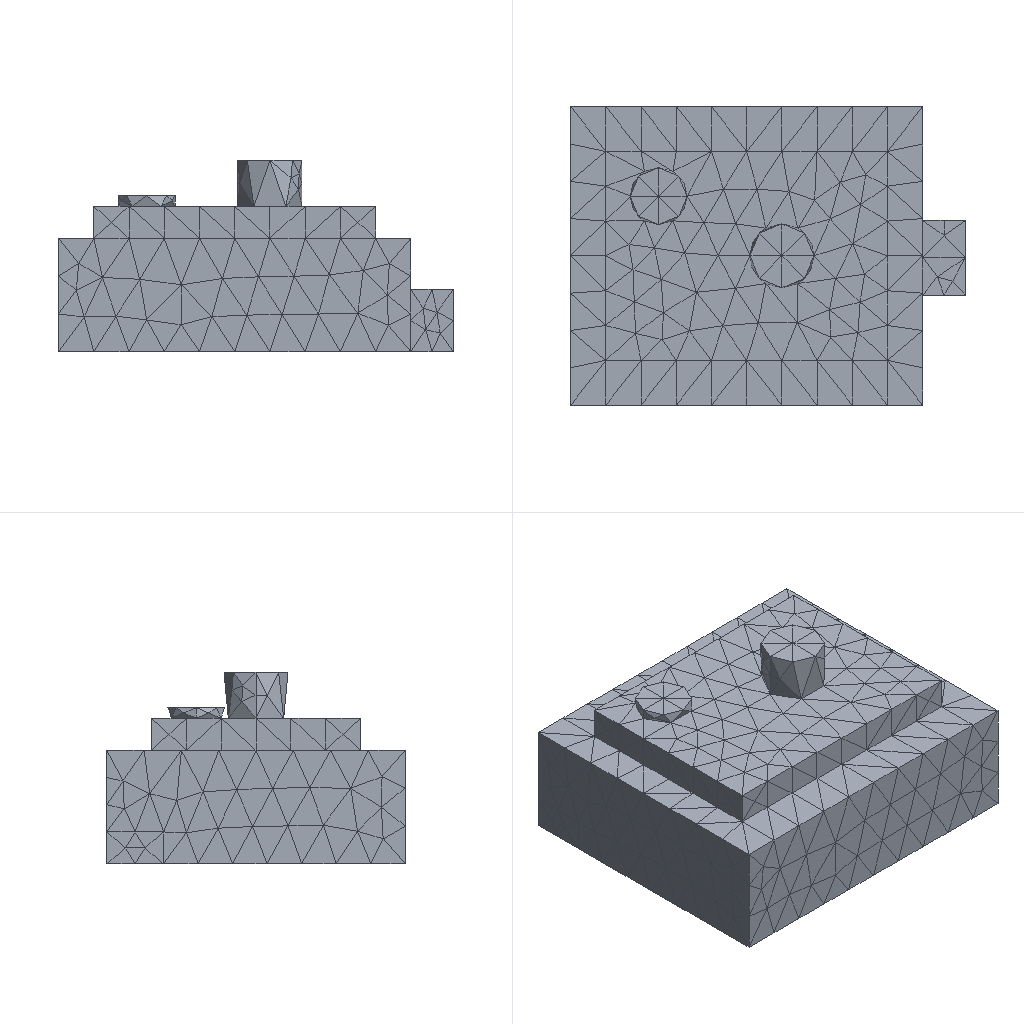Simulation study | ansys mapdl
Set-up summary:
category,name,step,type,value,unit,region
solver,ansys_mapdl
units,mm-N-s-tonne (MPa),,inferred,E=210000 density=
analysis,model,,static
mesh,nodes,,,4549
mesh,elements,,,2727
element_type,SOLID187,,,2727
material,mat 1,,E,210000
material,mat 1,,nu,0.3
load,,model,body load temp,,,all
load,,model,force,"1000 [dir=(0, 0, -1) n=148]",,node list
bc,,model,fixed,"[dofs=UX,UY,UZ n=4913]",,node list
Ansys APDL input file, long lists of numbers shortened:
/COM,ANSYS RELEASE 2026 R1           BUILD 26.1      UP20260202       09:08:28
/PREP7
/NOPR
/TITLE,2
ANTYPE, 0
*IF,_CDRDOFF,EQ,1,THEN     !if solid model was read in
_CDRDOFF=             !reset flag, numoffs already performed
*ELSE              !offset database for the following FE model
NUMOFF,NODE,     4549
NUMOFF,ELEM,     2727
NUMOFF,MAT ,        1
NUMOFF,TYPE,        1
*ENDIF
*SET,_RETURN ,  0.
*SET,_STATUS ,  0.
*SET,_UIQR   ,  148.
*SET,__FLOATPARAMETER__,  4549.
DOF,DELETE
ETBLOCK,        1,        1
(2i9,19a9)
        1      187        0        0        0        0        0        0        0        0        0        0        0        0        0        0        0        0        0        0        0
       -1
NBLOCK,6,SOLID,      4549,      4549
(3i9,6e21.13e3)
        1        0        0-3.3550000000000E+001 4.2000000000000E+001 9.0000000000000E+000
! (4548 more lines like these left out)
N,UNBL,LOC,       -1,
EBLOCK,19,SOLID,      2727,      2727
(19i10)
         1         1         1         1         0         0         0         0        10         0         1      1735      1736      1737      1738      1995      1996      1997      1998
! (5453 more lines like these left out)
        -1
MPTEMP,UNBL, 1, 1,  0.    ,
MPDATA,UNBL, 1,EX  ,       1, 1,  210000.000    ,
MPTEMP,UNBL, 1, 1,  0.    ,
MPDATA,UNBL, 1,NUXY,       1, 1, 0.3    ,
MPTEMP,UNBL, 1, 1,  0.    ,
MPDATA,UNBL, 1,PRXY,       1, 1, 0.3    ,
EXTOPT,ATTR,      0,      0,      0
EXTOPT,ESIZE,  0,  0.
EXTOPT,ACLEAR,      0
TREF,  0.
IRLF,  0
BFUNIF,TEMP,_TINY
ACEL,  0.    ,  0.    ,  0.
OMEGA,  0.    ,  0.    ,  0.
DOMEGA,  0.    ,  0.    ,  0.
CGLOC,  0.    ,  0.    ,  0.
CGOMEGA,  0.    ,  0.    ,  0.
DCGOMG,  0.    ,  0.    ,  0.
KUSE,     0
TIME,  0.
ALPHAD,  0.
BETAD,  0.
DMPRAT,  0.
DMPSTR,  0.
CRPLIM, 0.1    ,   0
CRPLIM,  0.    ,   1
NCNV,     0, 1.000000000E+12,     0,  0.    ,  0.
NEQIT,     0
ERESX,DEFA
DBLOCK,      4913
(i9,a6,2(pg16.9))
        1  UX    0.00000000      0.00000000
! (4912 more lines like these left out)
       -1
FBLOCK,       148
(i9,a6,2(pg16.9))
      872  FZ   -6.75675676      0.00000000
! (147 more lines like these left out)
       -1
/GO
FINISH
Results summary:
result,analysis_type_db,,,static,unstated
result,n_sets,,,1,unstated
result,load_steps[0].set,load_step=1,,1,unstated
result,load_steps[0].substep,load_step=1,,1,unstated
result,load_steps[0].time,load_step=1,,1,unstated
result,load_steps[0].freq,load_step=1,,1,unstated
result,load_steps[0].max_usum,load_step=1,,0.0004079,unstated
result,load_steps[0].max_seqv,load_step=1,,5.398,unstated
result,load_steps[0].reaction_sum.FX,load_step=1,,-9.3097e-12,unstated
result,load_steps[0].reaction_sum.FY,load_step=1,,-1.47992e-11,unstated
result,load_steps[0].reaction_sum.FZ,load_step=1,,1000,unstated
result,load_steps[0].reaction_sum.MX,load_step=1,,0,unstated
result,load_steps[0].reaction_sum.MY,load_step=1,,0,unstated
result,load_steps[0].reaction_sum.MZ,load_step=1,,0,unstated
result,convergence,,,results present for all listed sets,unstated